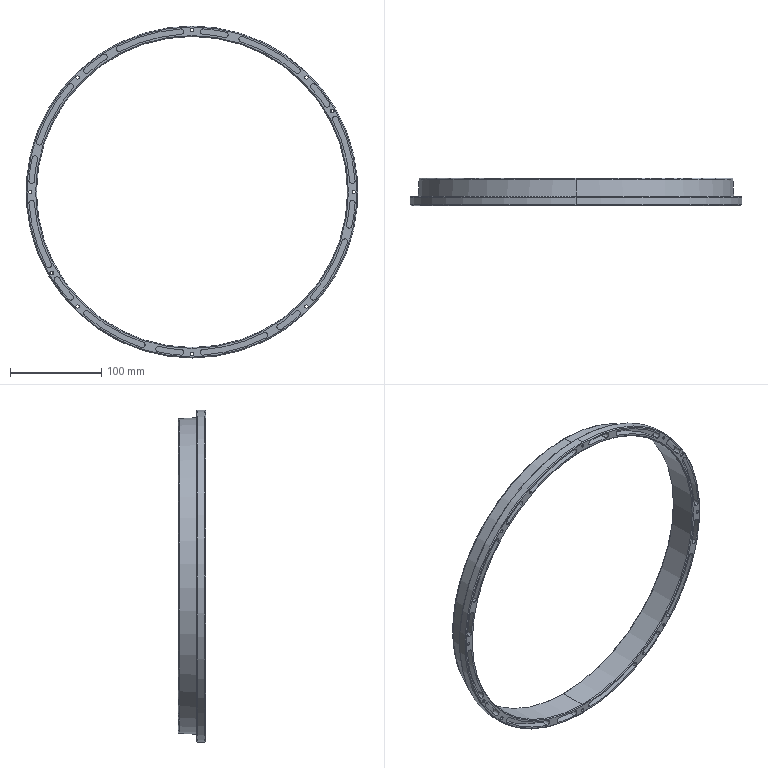Part | NX | features BREP 1 | 1 solid | 153 faces | box 363 x 30 x 363 mm | volume 137958 mm3 | cylinder 104 | cone 28 | plane 19 | torus 2 | commonest cylinder face diameters 6 x48 3.5 x16 345.5 x16 357.5 x16 3 x4 340 x2